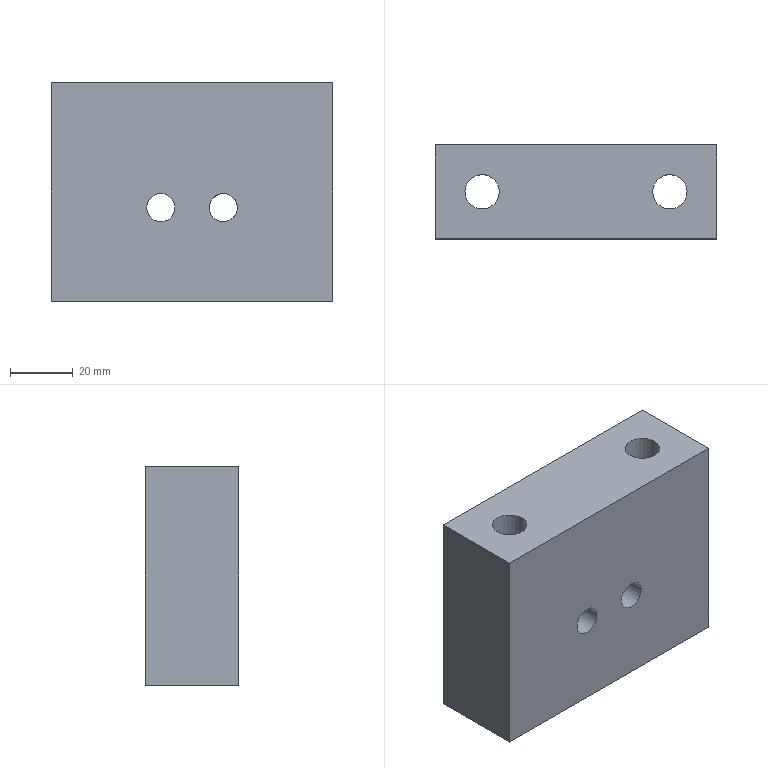Part | NX | features solid 2 | 1 solid | 18 faces | box 90 x 30 x 70 mm | volume 158613 mm3 | plane 10 | cylinder 8 | commonest cylinder face diameters 9 x2 11 x2 14 x2 17 x2
STEP:
#1=CARTESIAN_POINT('',(430.,-593.8,269.5));
#2=VERTEX_POINT('',#1);
#3=CARTESIAN_POINT('',(430.,-593.8,265.));
#4=DIRECTION('',(0.,1.,0.));
#5=DIRECTION('',(0.,0.,1.));
#6=AXIS2_PLACEMENT_3D('',#3,#4,#5);
#7=CIRCLE('',#6,4.5);
#8=EDGE_CURVE('',#2,#2,#7,.T.);
#9=ORIENTED_EDGE('',*,*,#8,.T.);
#10=EDGE_LOOP('',(#9));
#11=FACE_BOUND('',#10,.T.);
#12=CARTESIAN_POINT('',(410.,-593.8,269.5));
#13=VERTEX_POINT('',#12);
#14=CARTESIAN_POINT('',(410.,-593.8,265.));
#15=DIRECTION('',(0.,1.,0.));
#16=DIRECTION('',(0.,0.,1.));
#17=AXIS2_PLACEMENT_3D('',#14,#15,#16);
#18=CIRCLE('',#17,4.5);
#19=EDGE_CURVE('',#13,#13,#18,.T.);
#20=ORIENTED_EDGE('',*,*,#19,.T.);
#21=EDGE_LOOP('',(#20));
#22=FACE_BOUND('',#21,.T.);
#23=CARTESIAN_POINT('',(465.,-593.8,235.));
#24=VERTEX_POINT('',#23);
#25=CARTESIAN_POINT('',(465.,-593.8,305.));
#26=VERTEX_POINT('',#25);
#27=CARTESIAN_POINT('',(465.,-593.8,265.));
#28=DIRECTION('',(0.,0.,1.));
#29=VECTOR('',#28,1000.);
#30=LINE('',#27,#29);
#31=EDGE_CURVE('',#24,#26,#30,.T.);
#32=ORIENTED_EDGE('',*,*,#31,.T.);
#33=CARTESIAN_POINT('',(375.,-593.8,305.));
#34=VERTEX_POINT('',#33);
#35=CARTESIAN_POINT('',(10000360.,-593.8,305.));
#36=DIRECTION('',(-1.,0.,0.));
#37=VECTOR('',#36,1000.);
#38=LINE('',#35,#37);
#39=EDGE_CURVE('',#34,#26,#38,.F.);
#40=ORIENTED_EDGE('',*,*,#39,.F.);
#41=CARTESIAN_POINT('',(375.,-593.8,235.));
#42=VERTEX_POINT('',#41);
#43=CARTESIAN_POINT('',(375.,-593.8,265.));
#44=DIRECTION('',(0.,0.,-1.));
#45=VECTOR('',#44,1000.);
#46=LINE('',#43,#45);
#47=EDGE_CURVE('',#42,#34,#46,.F.);
#48=ORIENTED_EDGE('',*,*,#47,.F.);
#49=CARTESIAN_POINT('',(-9999530.,-593.8,235.));
#50=DIRECTION('',(1.,0.,0.));
#51=VECTOR('',#50,1000.);
#52=LINE('',#49,#51);
#53=EDGE_CURVE('',#42,#24,#52,.T.);
#54=ORIENTED_EDGE('',*,*,#53,.T.);
#55=EDGE_LOOP('',(#32,#40,#48,#54));
#56=FACE_BOUND('',#55,.T.);
#57=CARTESIAN_POINT('',(395.,-593.8,265.));
#58=DIRECTION('',(0.,-1.,0.));
#59=DIRECTION('',(1.,0.,0.));
#60=AXIS2_PLACEMENT_3D('',#57,#58,#59);
#61=PLANE('',#60);
#62=ADVANCED_FACE('',(#11,#22,#56),#61,.T.);
#63=ORIENTED_EDGE('',*,*,#47,.T.);
#64=CARTESIAN_POINT('',(375.,-563.8,305.));
#65=VERTEX_POINT('',#64);
#66=CARTESIAN_POINT('',(375.,-593.8,305.));
#67=DIRECTION('',(0.,1.,0.));
#68=VECTOR('',#67,1000.);
#69=LINE('',#66,#68);
#70=EDGE_CURVE('',#34,#65,#69,.T.);
#71=ORIENTED_EDGE('',*,*,#70,.T.);
#72=CARTESIAN_POINT('',(375.,-563.8,235.));
#73=VERTEX_POINT('',#72);
#74=CARTESIAN_POINT('',(375.,-563.8,265.));
#75=DIRECTION('',(0.,0.,1.));
#76=VECTOR('',#75,1000.);
#77=LINE('',#74,#76);
#78=EDGE_CURVE('',#73,#65,#77,.T.);
#79=ORIENTED_EDGE('',*,*,#78,.F.);
#80=CARTESIAN_POINT('',(375.,-593.8,235.));
#81=DIRECTION('',(0.,-1.,0.));
#82=VECTOR('',#81,1000.);
#83=LINE('',#80,#82);
#84=EDGE_CURVE('',#42,#73,#83,.F.);
#85=ORIENTED_EDGE('',*,*,#84,.F.);
#86=EDGE_LOOP('',(#63,#71,#79,#85));
#87=FACE_BOUND('',#86,.T.);
#88=CARTESIAN_POINT('',(375.,-593.8,265.));
#89=DIRECTION('',(1.,0.,0.));
#90=DIRECTION('',(0.,1.,0.));
#91=AXIS2_PLACEMENT_3D('',#88,#89,#90);
#92=PLANE('',#91);
#93=ADVANCED_FACE('',(#87),#92,.F.);
#94=CARTESIAN_POINT('',(430.,-563.8,272.));
#95=VERTEX_POINT('',#94);
#96=CARTESIAN_POINT('',(430.,-563.8,265.));
#97=DIRECTION('',(0.,1.,0.));
#98=DIRECTION('',(0.,0.,1.));
#99=AXIS2_PLACEMENT_3D('',#96,#97,#98);
#100=CIRCLE('',#99,7.);
#101=EDGE_CURVE('',#95,#95,#100,.F.);
#102=ORIENTED_EDGE('',*,*,#101,.T.);
#103=EDGE_LOOP('',(#102));
#104=FACE_BOUND('',#103,.T.);
#105=CARTESIAN_POINT('',(410.,-563.8,272.));
#106=VERTEX_POINT('',#105);
#107=CARTESIAN_POINT('',(410.,-563.8,265.));
#108=DIRECTION('',(0.,1.,0.));
#109=DIRECTION('',(0.,0.,1.));
#110=AXIS2_PLACEMENT_3D('',#107,#108,#109);
#111=CIRCLE('',#110,7.);
#112=EDGE_CURVE('',#106,#106,#111,.F.);
#113=ORIENTED_EDGE('',*,*,#112,.T.);
#114=EDGE_LOOP('',(#113));
#115=FACE_BOUND('',#114,.T.);
#116=ORIENTED_EDGE('',*,*,#78,.T.);
#117=CARTESIAN_POINT('',(465.,-563.8,305.));
#118=VERTEX_POINT('',#117);
#119=CARTESIAN_POINT('',(395.,-563.8,305.));
#120=DIRECTION('',(1.,0.,0.));
#121=VECTOR('',#120,1000.);
#122=LINE('',#119,#121);
#123=EDGE_CURVE('',#65,#118,#122,.T.);
#124=ORIENTED_EDGE('',*,*,#123,.T.);
#125=CARTESIAN_POINT('',(465.,-563.8,235.));
#126=VERTEX_POINT('',#125);
#127=CARTESIAN_POINT('',(465.,-563.8,265.));
#128=DIRECTION('',(0.,0.,-1.));
#129=VECTOR('',#128,1000.);
#130=LINE('',#127,#129);
#131=EDGE_CURVE('',#126,#118,#130,.F.);
#132=ORIENTED_EDGE('',*,*,#131,.F.);
#133=CARTESIAN_POINT('',(395.,-563.8,235.));
#134=DIRECTION('',(-1.,0.,0.));
#135=VECTOR('',#134,1000.);
#136=LINE('',#133,#135);
#137=EDGE_CURVE('',#73,#126,#136,.F.);
#138=ORIENTED_EDGE('',*,*,#137,.F.);
#139=EDGE_LOOP('',(#116,#124,#132,#138));
#140=FACE_BOUND('',#139,.T.);
#141=CARTESIAN_POINT('',(395.,-563.8,265.));
#142=DIRECTION('',(0.,-1.,0.));
#143=DIRECTION('',(1.,0.,0.));
#144=AXIS2_PLACEMENT_3D('',#141,#142,#143);
#145=PLANE('',#144);
#146=ADVANCED_FACE('',(#104,#115,#140),#145,.F.);
#147=CARTESIAN_POINT('',(465.,-10000637.8,235.));
#148=DIRECTION('',(0.,1.,0.));
#149=VECTOR('',#148,1000.);
#150=LINE('',#147,#149);
#151=EDGE_CURVE('',#24,#126,#150,.T.);
#152=ORIENTED_EDGE('',*,*,#151,.T.);
#153=ORIENTED_EDGE('',*,*,#131,.T.);
#154=CARTESIAN_POINT('',(465.,-10000637.8,305.));
#155=DIRECTION('',(0.,-1.,0.));
#156=VECTOR('',#155,1000.);
#157=LINE('',#154,#156);
#158=EDGE_CURVE('',#26,#118,#157,.F.);
#159=ORIENTED_EDGE('',*,*,#158,.F.);
#160=ORIENTED_EDGE('',*,*,#31,.F.);
#161=EDGE_LOOP('',(#152,#153,#159,#160));
#162=FACE_BOUND('',#161,.T.);
#163=CARTESIAN_POINT('',(465.,-593.8,265.));
#164=DIRECTION('',(1.,0.,0.));
#165=DIRECTION('',(0.,1.,0.));
#166=AXIS2_PLACEMENT_3D('',#163,#164,#165);
#167=PLANE('',#166);
#168=ADVANCED_FACE('',(#162),#167,.T.);
#169=CARTESIAN_POINT('',(395.5,-578.8,305.));
#170=VERTEX_POINT('',#169);
#171=CARTESIAN_POINT('',(390.,-578.8,305.));
#172=DIRECTION('',(0.,0.,-1.));
#173=DIRECTION('',(1.,0.,0.));
#174=AXIS2_PLACEMENT_3D('',#171,#172,#173);
#175=CIRCLE('',#174,5.5);
#176=EDGE_CURVE('',#170,#170,#175,.F.);
#177=ORIENTED_EDGE('',*,*,#176,.F.);
#178=EDGE_LOOP('',(#177));
#179=FACE_BOUND('',#178,.T.);
#180=CARTESIAN_POINT('',(455.5,-578.8,305.));
#181=VERTEX_POINT('',#180);
#182=CARTESIAN_POINT('',(450.,-578.8,305.));
#183=DIRECTION('',(0.,0.,-1.));
#184=DIRECTION('',(1.,0.,0.));
#185=AXIS2_PLACEMENT_3D('',#182,#183,#184);
#186=CIRCLE('',#185,5.5);
#187=EDGE_CURVE('',#181,#181,#186,.F.);
#188=ORIENTED_EDGE('',*,*,#187,.F.);
#189=EDGE_LOOP('',(#188));
#190=FACE_BOUND('',#189,.T.);
#191=ORIENTED_EDGE('',*,*,#123,.F.);
#192=ORIENTED_EDGE('',*,*,#70,.F.);
#193=ORIENTED_EDGE('',*,*,#39,.T.);
#194=ORIENTED_EDGE('',*,*,#158,.T.);
#195=EDGE_LOOP('',(#191,#192,#193,#194));
#196=FACE_BOUND('',#195,.T.);
#197=CARTESIAN_POINT('',(10000360.,-10000637.8,305.));
#198=DIRECTION('',(0.,0.,1.));
#199=DIRECTION('',(1.,0.,0.));
#200=AXIS2_PLACEMENT_3D('',#197,#198,#199);
#201=PLANE('',#200);
#202=ADVANCED_FACE('',(#179,#190,#196),#201,.T.);
#203=CARTESIAN_POINT('',(381.5,-578.8,235.));
#204=VERTEX_POINT('',#203);
#205=CARTESIAN_POINT('',(390.,-578.8,235.));
#206=DIRECTION('',(0.,0.,1.));
#207=DIRECTION('',(-1.,0.,0.));
#208=AXIS2_PLACEMENT_3D('',#205,#206,#207);
#209=CIRCLE('',#208,8.5);
#210=EDGE_CURVE('',#204,#204,#209,.T.);
#211=ORIENTED_EDGE('',*,*,#210,.T.);
#212=EDGE_LOOP('',(#211));
#213=FACE_BOUND('',#212,.T.);
#214=CARTESIAN_POINT('',(441.5,-578.8,235.));
#215=VERTEX_POINT('',#214);
#216=CARTESIAN_POINT('',(450.,-578.8,235.));
#217=DIRECTION('',(0.,0.,1.));
#218=DIRECTION('',(-1.,0.,0.));
#219=AXIS2_PLACEMENT_3D('',#216,#217,#218);
#220=CIRCLE('',#219,8.5);
#221=EDGE_CURVE('',#215,#215,#220,.T.);
#222=ORIENTED_EDGE('',*,*,#221,.T.);
#223=EDGE_LOOP('',(#222));
#224=FACE_BOUND('',#223,.T.);
#225=ORIENTED_EDGE('',*,*,#137,.T.);
#226=ORIENTED_EDGE('',*,*,#151,.F.);
#227=ORIENTED_EDGE('',*,*,#53,.F.);
#228=ORIENTED_EDGE('',*,*,#84,.T.);
#229=EDGE_LOOP('',(#225,#226,#227,#228));
#230=FACE_BOUND('',#229,.T.);
#231=CARTESIAN_POINT('',(-9999530.,-10000637.8,235.));
#232=DIRECTION('',(0.,0.,-1.));
#233=DIRECTION('',(-1.,0.,0.));
#234=AXIS2_PLACEMENT_3D('',#231,#232,#233);
#235=PLANE('',#234);
#236=ADVANCED_FACE('',(#213,#224,#230),#235,.T.);
#237=ORIENTED_EDGE('',*,*,#19,.F.);
#238=EDGE_LOOP('',(#237));
#239=FACE_BOUND('',#238,.T.);
#240=CARTESIAN_POINT('',(410.,-578.8,269.5));
#241=VERTEX_POINT('',#240);
#242=CARTESIAN_POINT('',(410.,-578.8,265.));
#243=DIRECTION('',(0.,1.,0.));
#244=DIRECTION('',(0.,0.,1.));
#245=AXIS2_PLACEMENT_3D('',#242,#243,#244);
#246=CIRCLE('',#245,4.5);
#247=EDGE_CURVE('',#241,#241,#246,.F.);
#248=ORIENTED_EDGE('',*,*,#247,.F.);
#249=EDGE_LOOP('',(#248));
#250=FACE_BOUND('',#249,.T.);
#251=CARTESIAN_POINT('',(410.,-578.8,265.));
#252=DIRECTION('',(0.,-1.,0.));
#253=DIRECTION('',(0.,0.,1.));
#254=AXIS2_PLACEMENT_3D('',#251,#252,#253);
#255=CYLINDRICAL_SURFACE('',#254,4.5);
#256=ADVANCED_FACE('',(#239,#250),#255,.F.);
#257=ORIENTED_EDGE('',*,*,#247,.T.);
#258=EDGE_LOOP('',(#257));
#259=FACE_BOUND('',#258,.T.);
#260=CARTESIAN_POINT('',(410.,-578.8,258.));
#261=VERTEX_POINT('',#260);
#262=CARTESIAN_POINT('',(410.,-578.8,265.));
#263=DIRECTION('',(0.,-1.,0.));
#264=DIRECTION('',(0.,0.,-1.));
#265=AXIS2_PLACEMENT_3D('',#262,#263,#264);
#266=CIRCLE('',#265,7.);
#267=EDGE_CURVE('',#261,#261,#266,.T.);
#268=ORIENTED_EDGE('',*,*,#267,.F.);
#269=EDGE_LOOP('',(#268));
#270=FACE_BOUND('',#269,.T.);
#271=CARTESIAN_POINT('',(410.,-578.8,265.));
#272=DIRECTION('',(0.,-1.,0.));
#273=DIRECTION('',(0.,0.,1.));
#274=AXIS2_PLACEMENT_3D('',#271,#272,#273);
#275=PLANE('',#274);
#276=ADVANCED_FACE('',(#259,#270),#275,.F.);
#277=ORIENTED_EDGE('',*,*,#112,.F.);
#278=EDGE_LOOP('',(#277));
#279=FACE_BOUND('',#278,.T.);
#280=ORIENTED_EDGE('',*,*,#267,.T.);
#281=EDGE_LOOP('',(#280));
#282=FACE_BOUND('',#281,.T.);
#283=CARTESIAN_POINT('',(410.,-578.8,265.));
#284=DIRECTION('',(0.,1.,0.));
#285=DIRECTION('',(0.,0.,-1.));
#286=AXIS2_PLACEMENT_3D('',#283,#284,#285);
#287=CYLINDRICAL_SURFACE('',#286,7.);
#288=ADVANCED_FACE('',(#279,#282),#287,.F.);
#289=ORIENTED_EDGE('',*,*,#8,.F.);
#290=EDGE_LOOP('',(#289));
#291=FACE_BOUND('',#290,.T.);
#292=CARTESIAN_POINT('',(425.5,-578.8,265.));
#293=VERTEX_POINT('',#292);
#294=CARTESIAN_POINT('',(430.,-578.8,265.));
#295=DIRECTION('',(0.,1.,0.));
#296=DIRECTION('',(-1.,0.,0.));
#297=AXIS2_PLACEMENT_3D('',#294,#295,#296);
#298=CIRCLE('',#297,4.5);
#299=EDGE_CURVE('',#293,#293,#298,.F.);
#300=ORIENTED_EDGE('',*,*,#299,.F.);
#301=EDGE_LOOP('',(#300));
#302=FACE_BOUND('',#301,.T.);
#303=CARTESIAN_POINT('',(430.,-578.8,265.));
#304=DIRECTION('',(0.,-1.,0.));
#305=DIRECTION('',(-1.,0.,0.));
#306=AXIS2_PLACEMENT_3D('',#303,#304,#305);
#307=CYLINDRICAL_SURFACE('',#306,4.5);
#308=ADVANCED_FACE('',(#291,#302),#307,.F.);
#309=ORIENTED_EDGE('',*,*,#299,.T.);
#310=EDGE_LOOP('',(#309));
#311=FACE_BOUND('',#310,.T.);
#312=CARTESIAN_POINT('',(437.,-578.8,265.));
#313=VERTEX_POINT('',#312);
#314=CARTESIAN_POINT('',(430.,-578.8,265.));
#315=DIRECTION('',(0.,-1.,0.));
#316=DIRECTION('',(1.,0.,0.));
#317=AXIS2_PLACEMENT_3D('',#314,#315,#316);
#318=CIRCLE('',#317,7.);
#319=EDGE_CURVE('',#313,#313,#318,.T.);
#320=ORIENTED_EDGE('',*,*,#319,.F.);
#321=EDGE_LOOP('',(#320));
#322=FACE_BOUND('',#321,.T.);
#323=CARTESIAN_POINT('',(430.,-578.8,265.));
#324=DIRECTION('',(0.,-1.,0.));
#325=DIRECTION('',(-1.,0.,0.));
#326=AXIS2_PLACEMENT_3D('',#323,#324,#325);
#327=PLANE('',#326);
#328=ADVANCED_FACE('',(#311,#322),#327,.F.);
#329=ORIENTED_EDGE('',*,*,#101,.F.);
#330=EDGE_LOOP('',(#329));
#331=FACE_BOUND('',#330,.T.);
#332=ORIENTED_EDGE('',*,*,#319,.T.);
#333=EDGE_LOOP('',(#332));
#334=FACE_BOUND('',#333,.T.);
#335=CARTESIAN_POINT('',(430.,-578.8,265.));
#336=DIRECTION('',(0.,1.,0.));
#337=DIRECTION('',(1.,0.,0.));
#338=AXIS2_PLACEMENT_3D('',#335,#336,#337);
#339=CYLINDRICAL_SURFACE('',#338,7.);
#340=ADVANCED_FACE('',(#331,#334),#339,.F.);
#341=CARTESIAN_POINT('',(455.5,-578.8,275.));
#342=VERTEX_POINT('',#341);
#343=CARTESIAN_POINT('',(450.,-578.8,275.));
#344=DIRECTION('',(0.,0.,-1.));
#345=DIRECTION('',(1.,0.,0.));
#346=AXIS2_PLACEMENT_3D('',#343,#344,#345);
#347=CIRCLE('',#346,5.5);
#348=EDGE_CURVE('',#342,#342,#347,.F.);
#349=ORIENTED_EDGE('',*,*,#348,.F.);
#350=EDGE_LOOP('',(#349));
#351=FACE_BOUND('',#350,.T.);
#352=ORIENTED_EDGE('',*,*,#187,.T.);
#353=EDGE_LOOP('',(#352));
#354=FACE_BOUND('',#353,.T.);
#355=CARTESIAN_POINT('',(450.,-578.8,335.));
#356=DIRECTION('',(0.,0.,-1.));
#357=DIRECTION('',(-1.,0.,0.));
#358=AXIS2_PLACEMENT_3D('',#355,#356,#357);
#359=CYLINDRICAL_SURFACE('',#358,5.5);
#360=ADVANCED_FACE('',(#351,#354),#359,.F.);
#361=ORIENTED_EDGE('',*,*,#348,.T.);
#362=EDGE_LOOP('',(#361));
#363=FACE_BOUND('',#362,.T.);
#364=CARTESIAN_POINT('',(441.5,-578.8,275.));
#365=VERTEX_POINT('',#364);
#366=CARTESIAN_POINT('',(450.,-578.8,275.));
#367=DIRECTION('',(0.,0.,1.));
#368=DIRECTION('',(-1.,0.,0.));
#369=AXIS2_PLACEMENT_3D('',#366,#367,#368);
#370=CIRCLE('',#369,8.5);
#371=EDGE_CURVE('',#365,#365,#370,.T.);
#372=ORIENTED_EDGE('',*,*,#371,.F.);
#373=EDGE_LOOP('',(#372));
#374=FACE_BOUND('',#373,.T.);
#375=CARTESIAN_POINT('',(450.,-578.8,275.));
#376=DIRECTION('',(0.,0.,1.));
#377=DIRECTION('',(1.,0.,0.));
#378=AXIS2_PLACEMENT_3D('',#375,#376,#377);
#379=PLANE('',#378);
#380=ADVANCED_FACE('',(#363,#374),#379,.F.);
#381=ORIENTED_EDGE('',*,*,#221,.F.);
#382=EDGE_LOOP('',(#381));
#383=FACE_BOUND('',#382,.T.);
#384=ORIENTED_EDGE('',*,*,#371,.T.);
#385=EDGE_LOOP('',(#384));
#386=FACE_BOUND('',#385,.T.);
#387=CARTESIAN_POINT('',(450.,-578.8,275.));
#388=DIRECTION('',(0.,0.,-1.));
#389=DIRECTION('',(-1.,0.,0.));
#390=AXIS2_PLACEMENT_3D('',#387,#388,#389);
#391=CYLINDRICAL_SURFACE('',#390,8.5);
#392=ADVANCED_FACE('',(#383,#386),#391,.F.);
#393=CARTESIAN_POINT('',(395.5,-578.8,275.));
#394=VERTEX_POINT('',#393);
#395=CARTESIAN_POINT('',(390.,-578.8,275.));
#396=DIRECTION('',(0.,0.,-1.));
#397=DIRECTION('',(1.,0.,0.));
#398=AXIS2_PLACEMENT_3D('',#395,#396,#397);
#399=CIRCLE('',#398,5.5);
#400=EDGE_CURVE('',#394,#394,#399,.F.);
#401=ORIENTED_EDGE('',*,*,#400,.F.);
#402=EDGE_LOOP('',(#401));
#403=FACE_BOUND('',#402,.T.);
#404=ORIENTED_EDGE('',*,*,#176,.T.);
#405=EDGE_LOOP('',(#404));
#406=FACE_BOUND('',#405,.T.);
#407=CARTESIAN_POINT('',(390.,-578.8,335.));
#408=DIRECTION('',(0.,0.,-1.));
#409=DIRECTION('',(-1.,0.,0.));
#410=AXIS2_PLACEMENT_3D('',#407,#408,#409);
#411=CYLINDRICAL_SURFACE('',#410,5.5);
#412=ADVANCED_FACE('',(#403,#406),#411,.F.);
#413=ORIENTED_EDGE('',*,*,#400,.T.);
#414=EDGE_LOOP('',(#413));
#415=FACE_BOUND('',#414,.T.);
#416=CARTESIAN_POINT('',(381.5,-578.8,275.));
#417=VERTEX_POINT('',#416);
#418=CARTESIAN_POINT('',(390.,-578.8,275.));
#419=DIRECTION('',(0.,0.,1.));
#420=DIRECTION('',(-1.,0.,0.));
#421=AXIS2_PLACEMENT_3D('',#418,#419,#420);
#422=CIRCLE('',#421,8.5);
#423=EDGE_CURVE('',#417,#417,#422,.T.);
#424=ORIENTED_EDGE('',*,*,#423,.F.);
#425=EDGE_LOOP('',(#424));
#426=FACE_BOUND('',#425,.T.);
#427=CARTESIAN_POINT('',(390.,-578.8,275.));
#428=DIRECTION('',(0.,0.,1.));
#429=DIRECTION('',(1.,0.,0.));
#430=AXIS2_PLACEMENT_3D('',#427,#428,#429);
#431=PLANE('',#430);
#432=ADVANCED_FACE('',(#415,#426),#431,.F.);
#433=ORIENTED_EDGE('',*,*,#210,.F.);
#434=EDGE_LOOP('',(#433));
#435=FACE_BOUND('',#434,.T.);
#436=ORIENTED_EDGE('',*,*,#423,.T.);
#437=EDGE_LOOP('',(#436));
#438=FACE_BOUND('',#437,.T.);
#439=CARTESIAN_POINT('',(390.,-578.8,275.));
#440=DIRECTION('',(0.,0.,-1.));
#441=DIRECTION('',(-1.,0.,0.));
#442=AXIS2_PLACEMENT_3D('',#439,#440,#441);
#443=CYLINDRICAL_SURFACE('',#442,8.5);
#444=ADVANCED_FACE('',(#435,#438),#443,.F.);
#445=CLOSED_SHELL('',(#62,#93,#146,#168,#202,#236,#256,#276,#288,#308,#328,#340,#360,#380,#392,#412,#432,#444));
#446=MANIFOLD_SOLID_BREP('',#445);
#447=(LENGTH_UNIT()NAMED_UNIT(*)SI_UNIT(.MILLI.,.METRE.));
#448=UNCERTAINTY_MEASURE_WITH_UNIT(LENGTH_MEASURE(0.00001),#447,'','');
#449=(NAMED_UNIT(*)PLANE_ANGLE_UNIT()SI_UNIT($,.RADIAN.));
#450=(NAMED_UNIT(*)SI_UNIT($,.STERADIAN.)SOLID_ANGLE_UNIT());
#451=(GEOMETRIC_REPRESENTATION_CONTEXT(3)GLOBAL_UNCERTAINTY_ASSIGNED_CONTEXT((#448))GLOBAL_UNIT_ASSIGNED_CONTEXT((#447,#449,#450))REPRESENTATION_CONTEXT('',''));
#452=ADVANCED_BREP_SHAPE_REPRESENTATION('',(#446),#451);